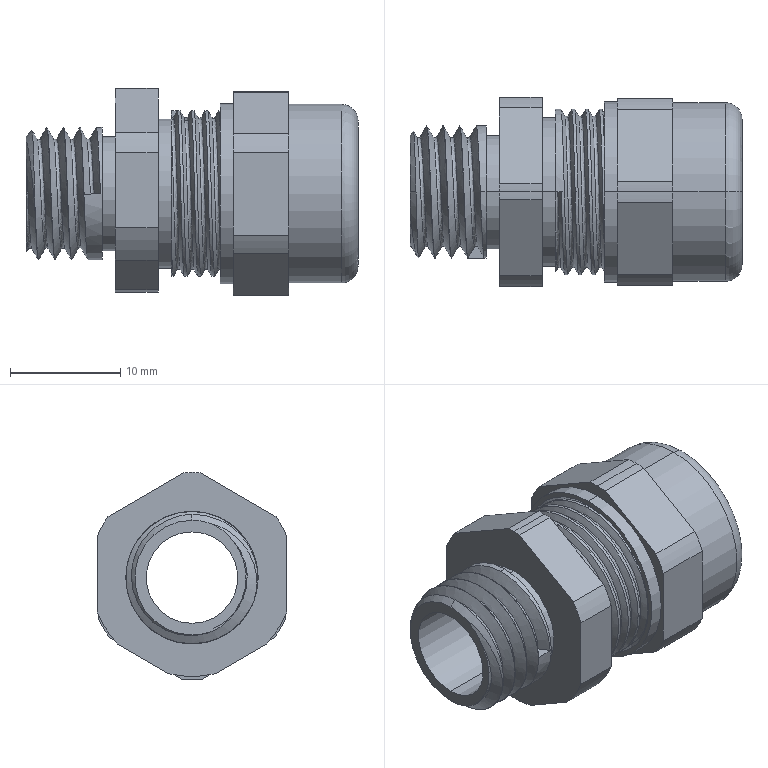Part | SolidWorks | features BaseBody 1 | 1 solid | 162 faces | box 30.12 x 17.2 x 18.788 mm | volume 3207 mm3 | plane 73 | cylinder 70 | cone 9 | spline 8 | torus 2 | commonest cylinder face diameters 13.5 x14 18.5 x14 14 x13 15 x9 12 x8 8.3 x2